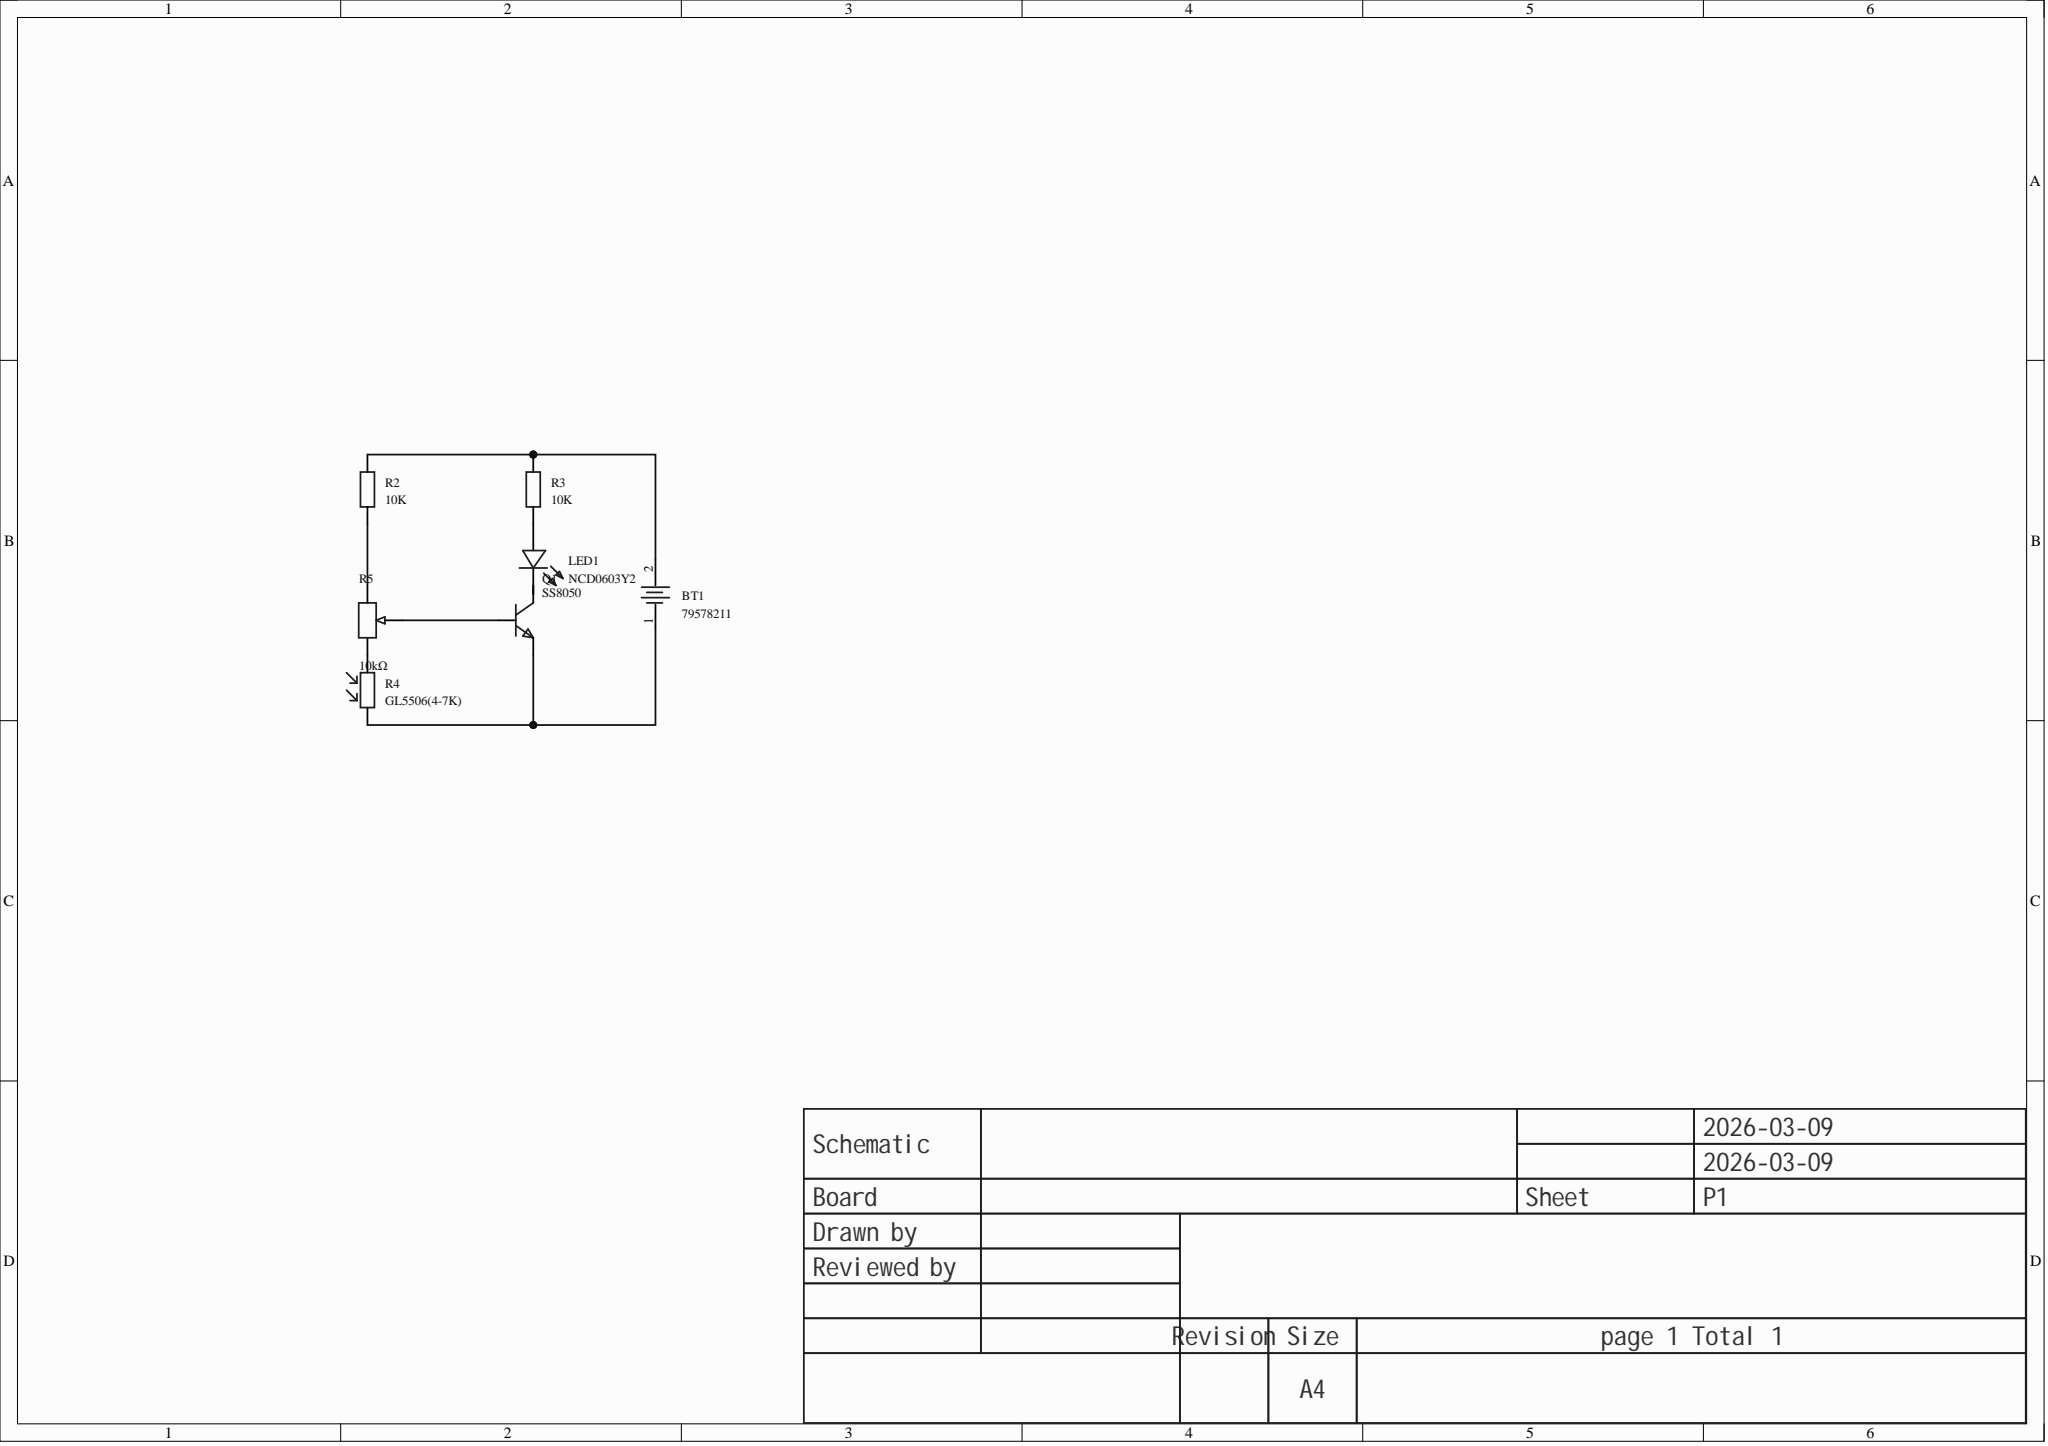Circuit board | Altium Designer | 7 parts | 7 nets
Bill of materials:
Comment,Description,Designator,Footprint,LibRef,Quantity
"79578211","","BT1","BAT-TH_79578211","79578211","1"
"NCD0603Y2","Emitted color: yellow; forward voltage (VF): 1.6V~2.6V; power: 65mW; forward current: 20mA; dominant wavelength: 586nm~595nm; lens color: colorless transparent lens; luminous intensity: 100mcd~220mcd; viewing angle: 130°; operating temperature: -30℃~+85℃;","LED1","LED0603-RD","NCD0603Y2","1"
"SS8050","Transistor type: NPN; collector current (Ic): 1.5A; collector-emitter breakdown voltage (Vceo): 25V; power dissipation (Pd): 300mW; DC current gain (hFE): 120@100mA,1.0V;","Q1","SOT-23-3_L2.9-W1.3-P1.90-LS2.4-BR","SS8050_C7420370","1"
"10K","","R2, R3","R0603","Res_0603","2"
"GL5506(4-7K)","Dark resistance: 500kΩ; light resistance @10Lux: 4kΩ~7kΩ; spectral peak (wavelength): 540nm;","R4","RES-TH_L5.1-W4.3-P3.00-D0.5","GL5506（4-7K）","1"
"10kΩ","Resistance: 10kΩ; tolerance: ±30%; power: -;","R5","RES-ADJ-TH_RDC1022A05","RDC1022A05","1"
Netlist (Protel format):
[
BT1
BAT-TH_79578211
79578211



]
[
LED1
LED0603-RD
NCD0603Y2



]
[
Q1
SOT-23-3_L2.9-W1.3-P1.90-LS2.4-BR
SS8050



]
[
R2
R0603
10K



]
[
R3
R0603
10K



]
[
R4
RES-TH_L5.1-W4.3-P3.00-D0.5
GL5506(4-7K)



]
[
R5
RES-ADJ-TH_RDC1022A05
10kΩ



]
(
NetR4_1
R4-1
R5-1
)
(
NetR2_1
R2-1
R5-3
)
(
NetQ1_1
Q1-1
R5-2
)
(
NetLED1_2
LED1-2
R3-1
)
(
NetLED1_1
LED1-1
Q1-3
)
(
NetBT1_2
BT1-2
R2-2
R3-2
)
(
NetBT1_1
BT1-1
Q1-2
R4-2
)